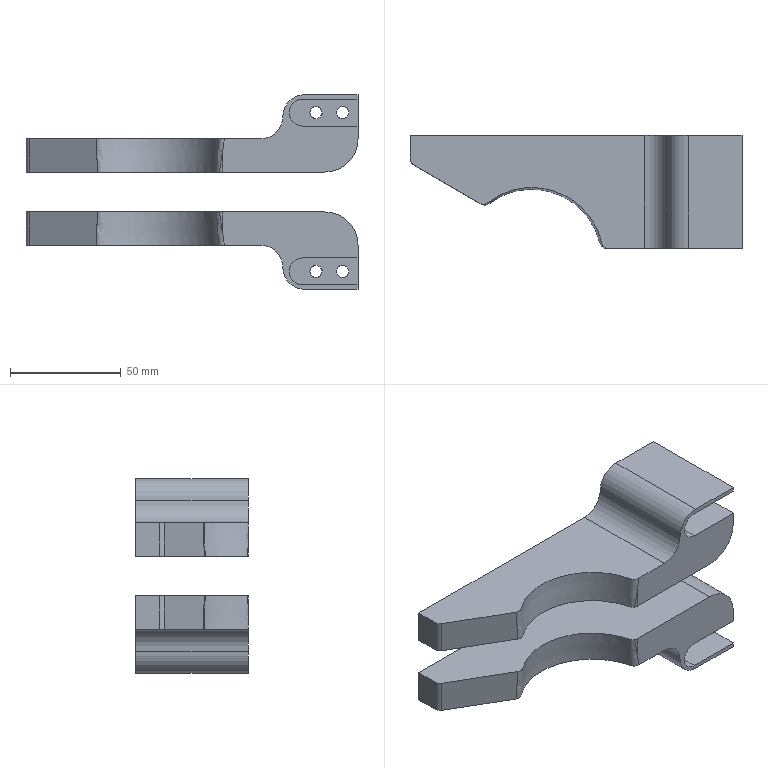NC program | NX | posted with a generic post | part box 150 x 51 x 88 mm
Lines 43 to 1093 of 21241:
(ADAPTIVE_MILLING , TOOL : D12C)
N72 T12 M6
N74 G54
N76 G17 G0 G90 X-87.244 Y-17.461 S9500 M3
N78 G43 Z30. H12
N80 Z-14.
N82 G94 G1 Z-17. F1000.
N84 X-85.489 Y-18.011 F3000.
N86 G3 X-84.077 Y-17.461 R1.22
N88 X-83.367 Y-14.688 R7.621
N90 X-83.032 Y-5.548 R92.487
N92 G1 X-83.024 Y-3.898
N94 X-83.019 Y-1.723
N96 X-83.015 Y1.652
N98 X-83.013 Y8.927
N100 X-83.012 Y17.177
N102 X-83.01 Y17.327
N104 G2 X-80.303 Y22.309 R6.799
N106 X-74.123 Y24.841 R13.407
N108 X-65.602 Y25.432 R57.013
N110 X-48.277 Y25.486 R906.104
N112 G1 X74.723 Y25.487
N114 X74.872 Y25.483
N116 X75.022 Y25.475
N118 X75.097 Y25.47
N120 G2 X80.104 Y22.371 R7.062
N122 X82.386 Y16.32 R14.219
N124 X82.935 Y7.945 R59.11
N126 G1 X82.948 Y7.045
N128 X82.959 Y5.92
N130 X82.968 Y4.57
N132 X82.976 Y2.77
N134 X82.982 Y0.445
N136 X82.986 Y-3.23
N138 X82.988 Y-12.155
N140 Y-17.18
N142 X82.986 Y-17.33
N144 X82.984 Y-17.405
N146 X82.98 Y-17.48
N148 X82.97 Y-17.629
N150 X82.963 Y-17.704
N152 G2 X79.846 Y-22.622 R7.111
N154 X73.789 Y-24.889 R14.27
N156 X65.189 Y-25.438 R61.879
N158 G1 X64.214 Y-25.45
N160 X63.089 Y-25.461
N162 X61.664 Y-25.47
N164 X59.789 Y-25.477
N166 X57.314 Y-25.482
N168 X53.189 Y-25.485
N170 X40.664 Y-25.486
N172 X-74.686 Y-25.485
N174 X-74.761
N176 X-74.836 Y-25.483
N178 X-74.986 Y-25.476
N180 X-75.135 Y-25.466
N182 G2 X-80.502 Y-21.496 R6.856
N184 X-81.891 Y-15.623 R15.41
N186 X-82.02 Y-5.5 R168.658
N188 G1 X-82.019 Y-3.4
N190 X-82.014 Y-1.526
N192 X-82.015 Y-0.851
N194 X-82.013 Y0.424
N196 Y0.799
N198 X-82.014 Y1.624
N200 X-82.013 Y2.674
N202 X-82.014 Y3.424
N204 X-82.012 Y4.624
N206 X-82.014 Y5.524
N208 X-82.012 Y6.349
N210 X-82.014 Y7.399
N212 X-82.012 Y8.149
N214 X-82.014 Y9.274
N216 X-82.011 Y10.249
N218 X-82.013 Y10.999
N220 X-82.011 Y12.124
N222 Y12.499
N224 G2 X-81.594 Y16.506 R11.873
N226 X-76.478 Y22.124 R9.91
N228 X-69.193 Y24.044 R20.954
N230 X-57.28 Y24.457 R127.664
N232 G1 X-55.405 Y24.465
N234 X-52.855 Y24.47
N236 X-48.805 Y24.473
N238 X-38.98 Y24.475
N240 X71.345
N242 X71.495 Y24.473
N244 G2 X75.124 Y23.638 R10.234
N246 X81.004 Y18.798 R6.219
N248 X81.925 Y5.12 R98.307
N250 X81.954 Y-14.454 R920.998
N252 X77.664 Y-21.409 R9.111
N254 X70.636 Y-23.852 R17.343
N256 X61.135 Y-24.423 R74.061
N258 G1 X60.085 Y-24.436
N260 X58.885 Y-24.447
N262 X57.385 Y-24.456
N264 X55.51 Y-24.464
N266 X53.035 Y-24.469
N268 X49.21 Y-24.473
N270 X40.51 Y-24.475
N272 X-71.315 Y-24.474
N274 X-71.54 Y-24.471
N276 X-71.689 Y-24.466
N278 X-71.839 Y-24.459
N280 G2 X-74.87 Y-23.669 R9.494
N282 X-77.568 Y-23.076 R7.913
N284 G1 X-76.435 Y-23.472
N286 X-76.298 Y-23.504
N288 X-74.958 Y-23.65
N290 G3 X-62.363 Y-23.866 R209.487
N292 G1 X-55.763 Y-23.867
N294 X53.437 Y-23.868
N296 X57.862 Y-23.849
N298 G3 X68.649 Y-23.421 R112.521
N300 X75.491 Y-21.581 R19.448
N302 X80.489 Y-15.157 R9.74
N304 X81.284 Y-8.47 R29.204
N306 X81.15 Y10.711 R329.089
N308 G1 Y17.465
N310 X81.146 Y17.535
N312 X81.15 Y17.465
N314 Y-2.479
N316 X81.149 Y-2.521
N318 X80.972 Y-5.218
N320 X80.961 Y-5.299
N322 G3 X80.24 Y-10.345 R50.96
N324 G2 X78.768 Y-15.664 R15.256
N326 X72.531 Y-20.915 R11.82
N328 X67.676 Y-22.181 R23.353
N330 G1 X65.529 Y-22.912
N332 X65.45 Y-22.933
N334 X62.819 Y-23.459
N336 X62.738 Y-23.469
N338 X60.041 Y-23.649
N340 X59.999 Y-23.65
N342 X-74.926
N344 G3 X-75.755 Y-25.717 R1.201
N346 X-75.12 Y-26.058 Z-16.97 R1.67
N348 G1 X-73.552 Y-26.64 Z-16.9
N350 X-71.389 Y-27.435
N352 X-71.107 Y-27.468
N354 X58.828
N356 G3 X62.934 Y-27.163 R28.578
N358 G1 X64.976 Y-26.858
N360 G3 X65.981 Y-25.91 R1.24
N362 G1 X66.707 Y-23.623 Z-17.
N364 X66.84 Y-23.199
N366 X66.989 Y-22.781
N368 G2 X67.676 Y-22.181 R1.23
N370 G3 X72.557 Y-20.132 R75.181
N372 X78.798 Y-12.537 R12.095
N374 G2 X79.555 Y-10.55 R7.79
N376 G1 X80.417 Y-8.01
N378 X80.438 Y-7.93
N380 X80.716 Y-6.533
N382 X80.417 Y-8.01
N384 X79.524 Y-10.626
N386 X78.338 Y-13.032
N388 X78.297 Y-13.104
N390 X76.807 Y-15.334
N392 X76.757 Y-15.4
N394 X74.99 Y-17.417
N396 X74.931 Y-17.475
N398 X72.916 Y-19.245
N400 X72.85 Y-19.295
N402 X70.621 Y-20.787
N404 X70.55 Y-20.828
N406 X68.263 Y-21.957
N408 G3 X68.819 Y-24.233 R1.201
N410 G1 X69.774 Y-24.092 Z-16.96
N412 X70.726 Y-23.925 Z-16.92
N414 X71.187 Y-23.847 Z-16.9
N416 X72.184 Y-23.685
N418 X73.177 Y-23.5
N420 X73.479 Y-23.355
N422 X75.216 Y-22.18
N424 G3 X76.991 Y-20.587 R12.992
N426 G1 X78.056 Y-19.428
N428 X79.108 Y-18.258
N430 G3 X83.669 Y-9.918 R23.949
N432 X84.453 Y-5.895 R22.965
N434 X84.701 Y-2.539 R45.859
N436 G1 X85.263 Y14.577
N438 G3 X84.268 Y20.632 R15.882
N440 G1 X83.73 Y22.018
N442 G3 X81.5 Y24.947 R8.257
N444 G1 X79.829 Y26.333
N446 G3 X78.081 Y26.113 R1.228
N448 G1 X76.466 Y24.338 Z-17.
N450 X76.037 Y23.889
N452 G2 X75.152 Y23.633 R1.23
N454 G3 X64.844 Y23.864 R148.205
N456 G1 X61.619 Y23.867
N458 X52.769 Y23.869
N460 X-53.506
N462 X-57.856 Y23.85
N464 G3 X-69.09 Y23.376 R105.485
N466 X-75.951 Y21.353 R18.214
N468 X-80.517 Y15.203 R9.723
N470 X-81.33 Y8.293 R29.495
N472 X-81.363 Y-13.231 R698.705
N474 X-81.15 Y-15.944 R43.884
N476 X-81.062 Y-18.28 R15.243
N478 G1 X-81.146 Y-17.535
N480 X-81.15 Y-17.465
N482 Y-2.535
N484 X-81.146 Y-2.465
N486 G2 X-80.696 Y0.865 R276.667
N488 G3 X-80.262 Y9.178 R362.735
N490 G2 X-79.133 Y14.89 R17.893
N492 X-73.254 Y20.614 R11.252
N494 X-65.331 Y22.465 R24.6
N496 X-51.84 Y22.848 R166.042
N498 G1 X-49.29 Y22.853
N500 X-45.09 Y22.856
N502 X-31.815 Y22.857
N504 X45.885
N506 X45.96 Y22.861
N508 X46.034 Y22.869
N510 X46.078 Y22.876
N512 X48.425 Y23.44
N514 X48.523 Y23.455
N516 X50.975 Y23.648
N518 X51.025 Y23.65
N520 X74.965
N522 G3 X75.789 Y25.722 R1.201
N524 X75.157 Y26.058 Z-16.97 R1.681
N526 G1 X73.584 Y26.642 Z-16.9
N528 X71.425 Y27.435
N530 X71.146 Y27.468
N532 X48.778 Y27.553
N534 G3 X47.602 Y26.614 R1.208
N536 G1 X47.541 Y26.341
N538 X47.018 Y23.999 Z-17.
N540 G2 X46.583 Y23.136 R1.419
N542 X46.078 Y22.876 R1.334
N544 X42.404 Y22.376 R14.027
N546 X27.105 Y22.264 R498.498
N548 G1 X-3.345
N550 X-3.72 Y22.262
N552 X-4.245 Y22.261
N554 X-4.845 Y22.259
N556 X-6.57 Y22.261
N558 X-7.095 Y22.259
N560 X-8.745 Y22.261
N562 X-9.345 Y22.259
N564 X-10.395 Y22.257
N566 X-11.37 Y22.256
N568 X-12.045 Y22.258
N570 X-12.87 Y22.256
N572 X-13.545 Y22.258
N574 X-14.37 Y22.256
N576 X-14.97 Y22.257
N578 X-15.72 Y22.256
N580 X-16.32 Y22.257
N582 X-17.07 Y22.256
N584 X-17.67 Y22.257
N586 X-18.42 Y22.256
N588 X-19.02 Y22.257
N590 X-19.77 Y22.256
N592 X-20.37 Y22.257
N594 X-21.12 Y22.256
N596 X-21.72 Y22.257
N598 X-22.47 Y22.256
N600 X-23.07 Y22.257
N602 X-23.82 Y22.256
N604 X-24.495 Y22.258
N606 X-25.32 Y22.256
N608 X-25.92 Y22.257
N610 X-26.67 Y22.256
N612 X-27.27 Y22.257
N614 X-28.02 Y22.256
N616 X-28.62 Y22.257
N618 X-29.37 Y22.256
N620 X-29.97 Y22.257
N622 X-30.72 Y22.256
N624 X-31.32 Y22.257
N626 X-32.145 Y22.256
N628 X-32.82 Y22.257
N630 X-33.645 Y22.256
N632 X-34.32 Y22.257
N634 X-35.22 Y22.256
N636 X-35.895 Y22.257
N638 X-36.72 Y22.256
N640 X-37.32 Y22.257
N642 X-38.145 Y22.256
N644 X-38.745 Y22.257
N646 G3 X-60.868 Y22.103 R769.766
N648 X-69.637 Y21.041 R41.206
N650 X-75.979 Y17.524 R13.101
N652 X-79.114 Y10.98 R13.326
N654 X-79.838 Y4.425 R48.391
N656 G2 X-80.194 Y0.771 R29.011
N658 G3 X-80.972 Y-1.065 R7.651
N660 G1 X-80.564 Y0.101
N662 X-80.503 Y0.228
N664 X-80.276 Y0.59
N666 G3 X-79.273 Y3.474 R7.619
N668 G2 X-78.254 Y9.614 R175.757
N670 X-74.256 Y16.742 R12.683
N672 X-67.071 Y20.133 R16.439
N674 X-57.386 Y21.119 R52.048
N676 X-34.587 Y21.255 R970.286
N678 G1 X-33.387 Y21.257
N680 X-32.487 Y21.255
N682 X-31.437 Y21.257
N684 X-30.537 Y21.256
N686 X-29.787 Y21.257
N688 X-28.887 Y21.255
N690 X-28.362 Y21.254
N692 X-27.612 Y21.256
N694 X-26.412 Y21.255
N696 X-25.737 Y21.254
N698 X-24.837 Y21.256
N700 X-23.712 Y21.255
N702 X-23.037 Y21.256
N704 X-22.062 Y21.255
N706 X-21.462 Y21.254
N708 X-20.637 Y21.256
N710 X-19.662 Y21.255
N712 X-18.912 Y21.257
N714 X-17.487 Y21.254
N716 X-16.812 Y21.255
N718 X-15.387
N720 X-14.487 Y21.254
N722 X-13.587 Y21.256
N724 X-12.687 Y21.255
N726 X-11.787 Y21.258
N728 X-10.812 Y21.257
N730 X-9.612 Y21.26
N732 X-8.412 Y21.258
N734 X-7.212 Y21.261
N736 X-6.387 Y21.26
N738 X-5.187 Y21.263
N740 X-4.212 Y21.261
N742 X-3.237 Y21.264
N744 X-2.487 Y21.263
N746 X-1.137 Y21.265
N748 X-0.687
N750 X-0.012 Y21.264
N752 X1.263 Y21.265
N754 X1.713 Y21.266
N756 X2.613 Y21.264
N758 X3.513 Y21.265
N760 X4.338 Y21.264
N762 X5.388 Y21.265
N764 X6.213 Y21.264
N766 X7.413 Y21.265
N768 X8.163 Y21.264
N770 X9.363 Y21.265
N772 X10.188 Y21.264
N774 X11.463 Y21.266
N776 X12.363 Y21.263
N778 X13.488 Y21.266
N780 X14.238 Y21.264
N782 X15.213 Y21.265
N784 X15.663 Y21.266
N786 X16.638 Y21.263
N788 X17.688 Y21.266
N790 X18.588 Y21.264
N792 X19.488 Y21.265
N794 X20.388 Y21.263
N796 X21.513 Y21.265
N798 X22.188 Y21.264
N800 X23.238 Y21.265
N802 X23.613 Y21.266
N804 X24.588 Y21.263
N806 X25.638 Y21.266
N808 X26.463 Y21.264
N810 X27.738 Y21.266
N812 G3 X42.061 Y21.422 R323.137
N814 X43.714 Y21.909 R2.573
N816 G1 X45.964 Y22.841
N818 X43.714 Y21.909
N820 X43.626 Y21.864
N822 X43.192 Y21.598
N824 G2 X40.886 Y20.996 R6.131
N826 X32.796 Y20.688 R80.456
N828 G1 X31.296 Y20.681
N830 X28.746 Y20.673
N832 X26.196 Y20.669
N834 X23.646
N836 X22.971 Y20.668
N838 X21.771
N840 X21.246
N842 X19.971 Y20.669
N844 X19.521 Y20.668
N846 X18.771 Y20.666
N848 X18.096 Y20.668
N850 X16.821 Y20.664
N852 X16.146 Y20.666
N854 X14.496 Y20.663
N856 X14.046 Y20.664
N858 X13.146 Y20.662
N860 X12.696 Y20.663
N862 X12.396
N864 X11.646 Y20.665
N866 X10.521 Y20.663
N868 X9.696 Y20.665
N870 X9.171
N872 X6.921 Y20.668
N874 X6.471 Y20.667
N876 X5.871
N878 X5.421
N880 X1.521 Y20.668
N882 X-2.379 Y20.666
N884 X-6.279 Y20.659
N886 X-6.429
N888 X-7.404 Y20.661
N890 X-8.004 Y20.659
N892 X-8.979 Y20.66
N894 X-10.404 Y20.656
N896 X-11.304 Y20.658
N898 X-12.204 Y20.655
N900 X-14.079 Y20.658
N902 X-15.054 Y20.655
N904 X-16.029 Y20.657
N906 X-17.229 Y20.654
N908 X-18.204 Y20.657
N910 X-18.729 Y20.655
N912 X-20.679 Y20.658
N914 X-21.504 Y20.656
N916 X-22.179
N918 X-22.629
N920 X-23.454 Y20.654
N922 X-24.954 Y20.657
N924 X-26.004 Y20.655
N926 X-27.504 Y20.658
N928 X-28.254 Y20.656
N930 X-29.229 Y20.658
N932 X-30.279 Y20.656
N934 X-30.729
N936 X-32.754 Y20.653
N938 X-33.204 Y20.654
N940 X-33.729 Y20.653
N942 X-34.629 Y20.655
N944 X-36.204 Y20.651
N946 X-36.954 Y20.653
N948 X-39.279 Y20.647
N950 X-39.654 Y20.648
N952 X-40.254 Y20.647
N954 X-40.704 Y20.646
N956 X-42.054 Y20.642
N958 X-42.654 Y20.643
N960 X-44.079 Y20.638
N962 X-44.679
N964 G3 X-59.974 Y20.373 R295.39
N966 X-68.386 Y18.983 R33.256
N968 X-77.082 Y10.262 R13.035
N970 X-78.538 Y4.137 R58.006
N972 G2 X-79.189 Y1.99 R9.577
N974 G3 X-79.926 Y1.147 R15.636
N976 G1 X-79.846 Y1.274
N978 X-79.758 Y1.385
N980 X-79.299 Y1.843
N982 G3 X-77.938 Y4.23 R5.766
N984 G2 X-76.2 Y9.42 R131.123
N986 X-67.788 Y17.559 R14.023
N988 X-58.986 Y19.277 R31.548
N990 X-45.568 Y19.618 R208.44
N992 G1 X-42.193 Y19.629
N994 X-38.443 Y19.638
N996 X-34.693 Y19.644
N998 X-32.743 Y19.645
N1000 X-32.143 Y19.648
N1002 X-30.268 Y19.652
N1004 X-28.393
N1006 X-26.818 Y19.65
N1008 X-25.993 Y19.653
N1010 X-24.943 Y19.652
N1012 X-23.968 Y19.655
N1014 X-22.768 Y19.653
N1016 X-22.018 Y19.655
N1018 X-21.268 Y19.654
N1020 X-20.668 Y19.653
N1022 X-19.618 Y19.655
N1024 X-18.343 Y19.653
N1026 X-17.293 Y19.656
N1028 X-16.093 Y19.654
N1030 X-14.968 Y19.657
N1032 X-13.693 Y19.654
N1034 X-12.868 Y19.656
N1036 X-11.743
N1038 X-10.618 Y19.659
N1040 X-9.868
N1042 X-8.368 Y19.66
N1044 X-7.393 Y19.663
N1046 X-6.643 Y19.662
N1048 X-5.518 Y19.664
N1050 X-4.693 Y19.663
N1052 X-3.718 Y19.666
N1054 X-2.893 Y19.665
N1056 X-1.918 Y19.667
N1058 X-1.168 Y19.666
N1060 X-0.193 Y19.668
N1062 X0.557 Y19.667
N1064 X1.532 Y19.668
N1066 X2.507 Y19.666
N1068 X3.707 Y19.669
N1070 X4.457 Y19.667
N1072 X5.582 Y19.668
N1074 X6.332 Y19.666
N1076 X7.307 Y19.667
N1078 X8.132 Y19.669
N1080 X9.107 Y19.665
N1082 X10.307 Y19.667
N1084 X11.207 Y19.665
N1086 X12.182
N1088 X13.382 Y19.663
N1090 X14.582 Y19.666
N1092 X15.332 Y19.665
N1094 X16.382 Y19.667
N1096 X16.907 Y19.668
N1098 X17.882 Y19.666
N1100 X18.632 Y19.668
N1102 X19.757 Y19.667
N1104 X20.207 Y19.666
N1106 X20.957 Y19.668
N1108 X22.157 Y19.666
N1110 X22.982 Y19.668
N1112 X23.882 Y19.667
N1114 G3 X38.204 Y19.85 R318.718
N1116 X41.023 Y20.215 R12.156
N1118 G1 X41.09 Y20.249
N1120 X41.156 Y20.285
N1122 X41.219 Y20.325
N1124 X41.239 Y20.336
N1126 X41.353 Y20.434
N1128 G2 X39.585 Y19.676 R3.473
N1130 X33.165 Y19.15 R37.386
N1132 X12.69 Y19.067 R954.501
N1134 G1 X10.065 Y19.069
N1136 X7.74 Y19.067
N1138 X7.515 Y19.066
N1140 X6.99 Y19.067
N1142 X6.69
N1144 X5.94 Y19.068
N1146 X5.115 Y19.066
N1148 X4.14 Y19.068
N1150 X2.865 Y19.066
N1152 X2.115 Y19.067
N1154 X1.065 Y19.065
N1156 X0.465 Y19.067
N1158 X-0.06 Y19.066
N1160 X-1.26 Y19.068
N1162 X-1.785 Y19.067
N1164 X-3.285 Y19.068
N1166 X-4.11 Y19.065
N1168 X-4.935 Y19.066
N1170 X-5.46 Y19.065
N1172 X-8.16 Y19.064
N1174 X-10.86 Y19.06
N1176 X-11.835 Y19.057
N1178 X-12.36 Y19.058
N1180 X-13.335 Y19.055
N1182 X-15.135 Y19.057
N1184 X-15.585 Y19.056
N1186 X-17.76 Y19.058
N1188 X-18.36 Y19.056
N1190 X-19.185 Y19.057
N1192 X-20.385 Y19.054
N1194 X-21.135 Y19.056
N1196 X-22.935 Y19.052
N1198 X-23.61 Y19.053
N1200 X-24.285 Y19.051
N1202 X-24.81 Y19.052
N1204 X-25.26 Y19.051
N1206 X-26.235 Y19.053
N1208 X-26.91 Y19.052
N1210 X-27.36 Y19.053
N1212 X-32.16 Y19.043
N1214 X-32.61 Y19.044
N1216 X-34.185 Y19.04
N1218 X-34.56 Y19.041
N1220 G3 X-55.258 Y18.852 R711.028
N1222 X-64.627 Y17.751 R47.076
N1224 X-72.265 Y13.663 R15.922
N1226 X-76.031 Y7.498 R17.955
N1228 G2 X-77.869 Y3.15 R38.279
N1230 X-78.774 Y2.346 R2.125
N1232 G1 X-78.885 Y2.258
N1234 X-79.044 Y2.099
N1236 X-78.885 Y2.258
N1238 X-78.774 Y2.346
N1240 X-78.261 Y2.669
N1242 G3 X-76.687 Y4.446 R4.74
N1244 G1 X-74.251 Y8.925
N1246 G2 X-64.593 Y16.298 R16.384
N1248 X-55.426 Y17.73 R39.445
N1250 X-39.155 Y18.017 R326.239
N1252 G1 X-34.43 Y18.029
N1254 X-31.58 Y18.034
N1256 X-30.98 Y18.038
N1258 X-29.555 Y18.043
N1260 X-28.13 Y18.044
N1262 X-27.455
N1264 X-26.555 Y18.048
N1266 X-25.505
N1268 X-24.38 Y18.052
N1270 X-23.555
N1272 X-22.205 Y18.054
N1274 X-21.755 Y18.055
N1276 X-21.155
N1278 X-20.03 Y18.057
N1280 X-19.655
N1282 X-18.681 Y18.055
N1284 X-17.781 Y18.057
N1286 X-16.881 Y18.055
N1288 X-16.506
N1290 X-15.681 Y18.056
N1292 X-14.406 Y18.055
N1294 X-13.281 Y18.059
N1296 X-12.381 Y18.058
N1298 X-11.406 Y18.061
N1300 X-10.656
N1302 X-9.306 Y18.064
N1304 X-8.856
N1306 X-8.181 Y18.063
N1308 X-6.831 Y18.067
N1310 X-6.381 Y18.068
N1312 X-5.781 Y18.067
N1314 X-4.431 Y18.068
N1316 X-3.906 Y18.069
N1318 X-3.081 Y18.067
N1320 X-2.106
N1322 X-1.206 Y18.066
N1324 X-0.456 Y18.067
N1326 X0.669 Y18.066
N1328 X1.419 Y18.067
N1330 X2.394 Y18.066
N1332 X3.369 Y18.068
N1334 X4.494 Y18.065
N1336 X5.769 Y18.069
N1338 X6.669 Y18.067
N1340 X7.719 Y18.069
N1342 X8.544 Y18.068
N1344 X9.669 Y18.069
N1346 X10.494 Y18.067
N1348 X11.694 Y18.069
N1350 X12.444 Y18.067
N1352 X13.419 Y18.068
N1354 X13.794
N1356 X14.769 Y18.066
N1358 X15.819 Y18.069
N1360 X16.644 Y18.067
N1362 X17.769 Y18.069
N1364 X18.444 Y18.068
N1366 X19.569 Y18.069
N1368 X20.094 Y18.07
N1370 X20.694 Y18.069
N1372 X21.894 Y18.071
N1374 X22.644 Y18.074
N1376 X23.244
N1378 G3 X35.915 Y18.315 R225.475
N1380 X39.461 Y18.879 R16.495
N1382 G1 X39.529 Y18.913
N1384 X39.594 Y18.95
N1386 X39.657 Y18.99
N1388 X39.701 Y19.023
N1390 X39.872 Y19.169
N1392 G2 X37.758 Y18.195 R4.206
N1394 X30.822 Y17.57 R37.583
N1396 X9.597 Y17.469 R966.703
N1398 G1 X8.172 Y17.471
N1400 X7.647 Y17.47
N1402 X7.272
N1404 X6.897 Y17.469
N1406 X5.772 Y17.47
N1408 X5.322 Y17.469
N1410 X3.747 Y17.47
N1412 X2.997 Y17.468
N1414 X2.172 Y17.469
N1416 X1.047 Y17.467
N1418 X0.447 Y17.468
N1420 X-0.603 Y17.466
N1422 X-1.353 Y17.468
N1424 X-2.253 Y17.466
N1426 X-2.703 Y17.467
N1428 X-3.378 Y17.466
N1430 X-4.203 Y17.468
N1432 X-5.178 Y17.465
N1434 X-5.703 Y17.466
N1436 X-6.003 Y17.465
N1438 X-6.528
N1440 X-7.353 Y17.463
N1442 X-7.803 Y17.464
N1444 X-8.478 Y17.462
N1446 X-9.153 Y17.463
N1448 X-9.828 Y17.46
N1450 X-10.653 Y17.461
N1452 X-12.228 Y17.457
N1454 X-13.353 Y17.458
N1456 X-14.253 Y17.456
N1458 X-14.928 Y17.457
N1460 X-16.278 Y17.455
N1462 X-16.878 Y17.456
N1464 X-19.053 Y17.453
N1466 X-19.428 Y17.454
N1468 X-20.403 Y17.452
N1470 X-20.928 Y17.453
N1472 X-21.528 Y17.451
N1474 X-22.128 Y17.452
N1476 X-23.028 Y17.449
N1478 X-24.228 Y17.45
N1480 X-25.053 Y17.447
N1482 X-25.653 Y17.448
N1484 X-26.103 Y17.447
N1486 X-26.778
N1488 X-31.353 Y17.432
N1490 X-31.803 Y17.433
N1492 X-33.078 Y17.428
N1494 X-33.528 Y17.429
N1496 X-35.478 Y17.422
N1498 X-35.928 Y17.423
N1500 G3 X-54.224 Y17.166 R438.121
N1502 X-63.63 Y15.805 R41.393
N1504 X-73.849 Y7.971 R17.179
N1506 G2 X-76.474 Y3.866 R53.531
N1508 X-77.728 Y3.003 R2.243
N1510 G1 X-78.046 Y2.804
N1512 X-77.728 Y3.003
N1514 X-77.601 Y3.064
N1516 X-77.222 Y3.197
N1518 G3 X-75.332 Y4.625 R4.326
N1520 G1 X-72.007 Y8.783
N1522 G2 X-61.682 Y14.946 R19.535
N1524 X-51.651 Y16.187 R50.333
N1526 X-31.254 Y16.429 R619.946
N1528 G1 X-30.729 Y16.431
N1530 X-30.054 Y16.435
N1532 X-29.079 Y16.437
N1534 X-28.404 Y16.44
N1536 X-27.504 Y16.441
N1538 X-26.304 Y16.44
N1540 X-25.254 Y16.446
N1542 X-24.354
N1544 X-23.379 Y16.449
N1546 X-22.254 Y16.447
N1548 X-21.429 Y16.45
N1550 X-20.304
N1552 X-19.704 Y16.452
N1554 X-18.504
N1556 X-17.829 Y16.454
N1558 X-16.704
N1560 X-16.029 Y16.455
N1562 X-14.979
N1564 X-14.079 Y16.457
N1566 X-12.954
N1568 X-12.054 Y16.459
N1570 X-11.154
N1572 X-10.404 Y16.461
N1574 X-9.204 Y16.46
N1576 X-8.454 Y16.462
N1578 X-6.804 Y16.46
N1580 X-5.829 Y16.463
N1582 X-5.154
N1584 X-4.554
N1586 X-3.954 Y16.464
N1588 X-2.754
N1590 X-2.079 Y16.466
N1592 X-1.104 Y16.465
N1594 X-0.504 Y16.466
N1596 X0.771
N1598 X1.446 Y16.468
N1600 X2.571 Y16.467
N1602 X3.321 Y16.469
N1604 X4.596 Y16.467
N1606 X5.271 Y16.468
N1608 X6.546
N1610 X7.071 Y16.467
N1612 X7.671 Y16.468
N1614 X8.721
N1616 X9.471 Y16.47
N1618 X10.446 Y16.469
N1620 X11.346 Y16.472
N1622 X12.396 Y16.47
N1624 X13.221 Y16.472
N1626 X14.121 Y16.471
N1628 X15.396 Y16.475
N1630 X16.296 Y16.473
N1632 G3 X32.868 Y16.694 R368.96
N1634 X38.183 Y17.547 R20.109
N1636 X38.751 Y17.949 R1.745
N1638 G2 X37.037 Y16.934 R3.271
N1640 X31.338 Y16.096 R23.833
N1642 X17.316 Y15.883 R324.782
N1644 G1 X6.591 Y15.866
N1646 X5.691 Y15.868
N1648 X5.016 Y15.866
N1650 X3.816 Y15.868
N1652 X3.216 Y15.867
N1654 X1.791 Y15.869
N1656 X1.266 Y15.868
N1658 X0.441 Y15.869
N1660 X-0.609 Y15.866
N1662 X-2.109 Y15.863
N1664 X-3.459 Y15.865
N1666 X-4.284 Y15.863
N1668 X-5.334 Y15.864
N1670 X-5.859 Y15.863
N1672 X-6.234 Y15.864
N1674 X-6.834 Y15.862
N1676 X-7.434 Y15.863
N1678 X-8.859 Y15.859
N1680 X-10.734 Y15.856
N1682 X-11.259
N1684 X-11.484
N1686 X-11.784
N1688 X-12.609 Y15.855
N1690 X-13.059
N1692 X-13.884
N1694 X-14.334
N1696 X-14.784 Y15.856
N1698 X-16.284 Y15.852
N1700 X-18.009 Y15.849
N1702 X-18.834 Y15.851
N1704 X-19.659 Y15.849
N1706 X-21.084 Y15.851
N1708 X-21.609 Y15.85
N1710 X-23.334
N1712 X-24.009 Y15.847
N1714 X-25.059
N1716 X-25.584 Y15.844
N1718 X-26.184
N1720 X-26.709 Y15.842
N1722 X-27.084
N1724 X-41.709 Y15.779
N1726 X-43.734 Y15.759
N1728 X-45.608 Y15.738
N1730 G3 X-57.58 Y15.035 R99.257
N1732 X-66.665 Y12.125 R24.76
N1734 X-72.792 Y6.665 R23.578
N1736 G2 X-75.649 Y3.703 R19.592
N1738 X-76.435 Y3.472 R2.503
N1740 G1 X-77.002 Y3.274
N1742 X-76.435 Y3.472
N1744 X-76.298 Y3.504
N1746 X-76.082 Y3.528
N1748 G3 X-74.148 Y4.451 R3.734
N1750 X-70.485 Y7.777 R79.262
N1752 G2 X-58.224 Y13.684 R24.038
N1754 X-46.953 Y14.659 R72.934
N1756 X-25.729 Y14.836 R975.343
N1758 G1 X-23.029 Y14.847
N1760 X-22.354
N1762 X-21.079 Y14.849
N1764 X-20.179 Y14.848
N1766 X-19.204 Y14.85
N1768 X-18.529
N1770 X-17.404 Y14.853
N1772 X-16.279 Y14.851
N1774 X-15.604 Y14.853
N1776 X-14.329 Y14.852
N1778 X-13.804
N1780 X-12.979 Y14.855
N1782 X-11.779 Y14.854
N1784 X-10.729 Y14.858
N1786 X-9.604
N1788 X-8.554 Y14.861
N1790 X-7.354 Y14.859
N1792 X-6.454 Y14.862
N1794 X-5.554 Y14.861
N1796 X-5.179
N1798 X-3.979 Y14.864
N1800 X-3.154 Y14.863
N1802 X-2.254 Y14.866
N1804 X-1.504 Y14.865
N1806 X-0.829 Y14.864
N1808 X-0.154 Y14.865
N1810 X1.271
N1812 X1.946 Y14.864
N1814 X2.771 Y14.866
N1816 X3.896 Y14.865
N1818 X4.796 Y14.867
N1820 X5.696 Y14.866
N1822 X6.821 Y14.869
N1824 X7.496 Y14.868
N1826 G3 X29.095 Y15.038 R779.688
N1828 X36.009 Y15.836 R32.277
N1830 X37.586 Y16.5 R4.002
N1832 G1 X37.638 Y16.554
N1834 X37.688 Y16.61
N1836 X37.719 Y16.641
N1838 X37.908 Y16.95
N1840 X37.967 Y17.03
N1842 X38.113 Y17.202
N1844 X37.967 Y17.03
N1846 X37.908 Y16.95
N1848 X37.719 Y16.641
N1850 G2 X36.117 Y15.594 R3.223
N1852 X30.526 Y14.589 R20.753
N1854 X16.806 Y14.291 R229.278
N1856 G1 X14.481 Y14.28
N1858 X13.731
N1860 X12.606 Y14.276
N1862 X11.406 Y14.277
N1864 X10.131 Y14.272
N1866 X9.006
N1868 X8.106 Y14.269
N1870 X7.506 Y14.27
N1872 X6.231 Y14.266
N1874 X5.556 Y14.267
N1876 X4.206 Y14.264
N1878 X2.706 Y14.267
N1880 X1.581 Y14.264
N1882 X1.056
N1884 X-1.569 Y14.262
N1886 X-4.194 Y14.264
N1888 X-5.019 Y14.261
N1890 X-5.769 Y14.263
N1892 X-7.719 Y14.258
N1894 X-8.319 Y14.259
N1896 X-9.369 Y14.256
N1898 X-10.719 Y14.257
N1900 X-11.169 Y14.256
N1902 X-16.494
N1904 X-17.394
N1906 X-17.919 Y14.254
N1908 X-18.669
N1910 X-19.569 Y14.251
N1912 X-20.769
N1914 X-35.244 Y14.195
N1916 X-36.144 Y14.188
N1918 X-36.669 Y14.186
N1920 X-41.693 Y14.144
N1922 G3 X-54.723 Y13.533 R130.639
N1924 X-64.726 Y10.794 R29.718
N1926 X-71.124 Y6.244 R29.833
N1928 G2 X-74.408 Y3.763 R18.606
N1930 X-75.93 Y3.545 R7.092
N1932 G1 X-75.035 Y3.646
N1934 X-74.965 Y3.65
N1936 X-74.852
N1938 G3 X-72.6 Y4.379 R4.234
N1940 X-68.083 Y7.469 R96.847
N1942 G2 X-55.28 Y12.275 R29.674
N1944 X-42.865 Y13.088 R98.821
N1946 X-27.641 Y13.212 R799.672
N1948 G1 X-16.541 Y13.256
N1950 X-15.416 Y13.254
N1952 X-14.741 Y13.255
N1954 X-13.466 Y13.254
N1956 X-13.091
N1958 X-11.666 Y13.258
N1960 X-10.916 Y13.257
N1962 X-9.791 Y13.259
N1964 X-9.041 Y13.261
N1966 X-8.066 Y13.26
N1968 X-7.241 Y13.261
N1970 X-5.966
N1972 X-5.291 Y13.26
N1974 X-4.616 Y13.261
N1976 X-3.341 Y13.26
N1978 X-2.216 Y13.263
N1980 X-1.391 Y13.262
N1982 X-0.641 Y13.264
N1984 X-0.191 Y13.265
N1986 X1.084 Y13.263
N1988 X2.359 Y13.267
N1990 X3.259 Y13.265
N1992 X4.159 Y13.267
N1994 X4.534 Y13.268
N1996 X5.284
N1998 X6.409 Y13.27
N2000 X7.384
N2002 X8.434 Y13.273
N2004 X9.184
N2006 X9.634 Y13.272
N2008 G3 X28.006 Y13.491 R517.12
N2010 X34.906 Y14.401 R30.674
N2012 X36.867 Y15.301 R5.038
N2014 G1 X36.917 Y15.357
N2016 X36.964 Y15.415
N2018 X36.989 Y15.45
N2020 X37.106 Y15.641
N2022 G2 X35.59 Y14.363 R2.876
N2024 X30.352 Y13.148 R17.105
N2026 X18.289 Y12.715 R134.665
N2028 G1 X16.639 Y12.705
N2030 X15.739 Y12.701
N2032 X15.214 Y12.696
N2034 X13.04 Y12.688
N2036 X12.74
N2038 X12.29 Y12.684
N2040 X10.865 Y12.682
N2042 X10.34 Y12.679
N2044 X-6.085 Y12.658
N2046 X-6.685 Y12.659
N2048 X-8.11 Y12.656
N2050 X-9.31 Y12.659
N2052 X-10.435 Y12.655
N2054 X-12.31 Y12.658
N2056 X-13.06 Y12.656
N2058 X-13.885 Y12.657
N2060 X-18.16 Y12.643
N2062 X-28.21 Y12.603
N2064 X-35.26 Y12.573
N2066 X-37.885 Y12.548
N2068 G3 X-52.195 Y11.996 R165.864
N2070 X-62.95 Y9.44 R35.772
N2072 X-69.257 Y5.837 R38.285
N2074 G2 X-73.029 Y3.691 R19.143
N2076 X-74.626 Y3.65 R12.093
N2078 G1 X-73.276
N2080 G3 X-70.405 Y4.405 R6.051
N2082 X-64.969 Y7.279 R740.093
N2084 G2 X-51.511 Y10.932 R38.321
N2086 X-37.503 Y11.529 R161.802
N2088 G1 X-36.003 Y11.546
N2090 X-34.503 Y11.559
N2092 X-33.003 Y11.569
N2094 X-28.503 Y11.59
N2096 X-20.628 Y11.622
N2098 X-12.078 Y11.652
N2100 X-9.753 Y11.66
N2102 X-9.078 Y11.658
N2104 X-7.653 Y11.659
N2106 X-6.828 Y11.661
N2108 X-6.228 Y11.66
N2110 X-5.028 Y11.662
N2112 X-4.578 Y11.663
N2114 X-3.678 Y11.662
N2116 X-2.553 Y11.665
N2118 X-1.878 Y11.664
N2120 X-0.603 Y11.667
N2122 X-0.153 Y11.668
N2124 X0.522 Y11.667
N2126 X1.572 Y11.67
N2128 X2.097
N2130 X2.772 Y11.669
N2132 X3.597 Y11.671
N2134 X4.647
N2136 X5.472 Y11.673
N2138 G3 X25.944 Y11.891 R599.686
N2140 X33.521 Y12.831 R36.233
N2142 X36.175 Y14.01 R7.023
N2144 X36.636 Y14.874 R3.298
N2146 G1 X36.793 Y15.13
N2148 X36.636 Y14.874
N2150 X36.591 Y14.786
N2152 X36.405 Y14.337
N2154 G2 X35.252 Y13.206 R2.331
N2156 X30.315 Y11.753 R14.316
N2158 X19.689 Y11.158 R88.073
N2160 X-0.411 Y11.069 R976.003
N2162 G1 X-1.461 Y11.065
N2164 X-2.286 Y11.066
N2166 X-2.736 Y11.065